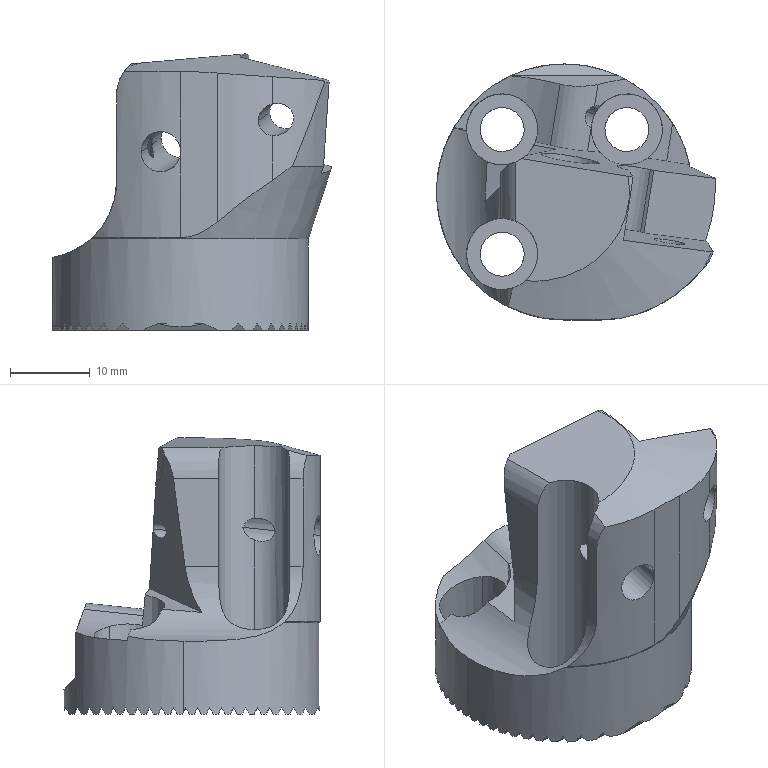NC program | Mastercam | posted with a generic post
Lines 5249 to 6702 of 7888:
(4 FEMR |TOOL - 6|DIA. OFF. - 6|LEN. - 6|TOOL DIA. - 4.)
N652 T6 M6
N654 G0 G54 G90 X24.079 Y12.972 C9. B-84. S3500 M3
N656 G43 H6 Z56.807
N658 Z7.807
N660 G1 Z6.607 F2000.
N662 G41 D6 X23.527 Y12.824 F400.
N664 G3 X23.484 Y12.769 I.014 J-.055
N666 X23.486 Y12.754 I.057
N668 G1 X23.917 Y11.146
N670 G2 X23.987 Y10.616 I-1.98 J-.53
N672 X23.616 Y9.44 I-2.05
N674 G1 X23.314 Y9.009
N676 G3 X23.196 Y8.636 I.533 J-.373
N678 X23.847 Y7.985 I.651
N680 X24.379 Y8.263 J.651
N682 G1 X24.681 Y8.694
N684 G2 X26.182 Y9.56 I1.679 J-1.176
N686 G1 X27.875 Y9.709
N688 G3 X27.926 Y9.765 I-.005 J.056
N690 G1 Y9.77
N692 G40 X27.877 Y10.34
N694 X24.079 Y12.972
N696 Z6.407 F2000.
N698 G41 D6 X23.527 Y12.824 F400.
N700 G3 X23.484 Y12.769 I.014 J-.055
N702 X23.486 Y12.754 I.057
N704 G1 X23.917 Y11.146
N706 G2 X23.987 Y10.616 I-1.98 J-.53
N708 X23.616 Y9.44 I-2.05
N710 G1 X23.314 Y9.009
N712 G3 X23.196 Y8.636 I.533 J-.373
N714 X23.847 Y7.985 I.651
N716 X24.379 Y8.263 J.651
N718 G1 X24.681 Y8.694
N720 G2 X26.182 Y9.56 I1.679 J-1.176
N722 G1 X27.875 Y9.709
N724 G3 X27.926 Y9.765 I-.005 J.056
N726 G1 Y9.77
N728 G40 X27.877 Y10.34
N730 X24.079 Y12.972
N732 Z6.207 F2000.
N734 G41 D6 X23.527 Y12.824 F400.
N736 G3 X23.484 Y12.769 I.014 J-.055
N738 X23.486 Y12.754 I.057
N740 G1 X23.917 Y11.146
N742 G2 X23.987 Y10.616 I-1.98 J-.53
N744 X23.616 Y9.44 I-2.05
N746 G1 X23.314 Y9.009
N748 G3 X23.196 Y8.636 I.533 J-.373
N750 X23.847 Y7.985 I.651
N752 X24.379 Y8.263 J.651
N754 G1 X24.681 Y8.694
N756 G2 X26.182 Y9.56 I1.679 J-1.176
N758 G1 X27.875 Y9.709
N760 G3 X27.926 Y9.765 I-.005 J.056
N762 G1 Y9.77
N764 G40 X27.877 Y10.34
N766 X24.079 Y12.972
N768 Z6.007 F2000.
N770 G41 D6 X23.527 Y12.824 F400.
N772 G3 X23.484 Y12.769 I.014 J-.055
N774 X23.486 Y12.754 I.057
N776 G1 X23.917 Y11.146
N778 G2 X23.987 Y10.616 I-1.98 J-.53
N780 X23.616 Y9.44 I-2.05
N782 G1 X23.314 Y9.009
N784 G3 X23.196 Y8.636 I.533 J-.373
N786 X23.847 Y7.985 I.651
N788 X24.379 Y8.263 J.651
N790 G1 X24.681 Y8.694
N792 G2 X26.182 Y9.56 I1.679 J-1.176
N794 G1 X27.875 Y9.709
N796 G3 X27.926 Y9.765 I-.005 J.056
N798 G1 Y9.77
N800 G40 X27.877 Y10.34
N802 X24.079 Y12.972
N804 Z5.807 F2000.
N806 G41 D6 X23.527 Y12.824 F400.
N808 G3 X23.484 Y12.769 I.014 J-.055
N810 X23.486 Y12.754 I.057
N812 G1 X23.917 Y11.146
N814 G2 X23.987 Y10.616 I-1.98 J-.53
N816 X23.616 Y9.44 I-2.05
N818 G1 X23.314 Y9.009
N820 G3 X23.196 Y8.636 I.533 J-.373
N822 X23.847 Y7.985 I.651
N824 X24.379 Y8.263 J.651
N826 G1 X24.681 Y8.694
N828 G2 X26.182 Y9.56 I1.679 J-1.176
N830 G1 X27.875 Y9.709
N832 G3 X27.926 Y9.765 I-.005 J.056
N834 G1 Y9.77
N836 G40 X27.877 Y10.34
N838 X24.079 Y12.972
N840 Z5.607 F2000.
N842 G41 D6 X23.527 Y12.824 F400.
N844 G3 X23.484 Y12.769 I.014 J-.055
N846 X23.486 Y12.754 I.057
N848 G1 X23.917 Y11.146
N850 G2 X23.987 Y10.616 I-1.98 J-.53
N852 X23.616 Y9.44 I-2.05
N854 G1 X23.314 Y9.009
N856 G3 X23.196 Y8.636 I.533 J-.373
N858 X23.847 Y7.985 I.651
N860 X24.379 Y8.263 J.651
N862 G1 X24.681 Y8.694
N864 G2 X26.182 Y9.56 I1.679 J-1.176
N866 G1 X27.875 Y9.709
N868 G3 X27.926 Y9.765 I-.005 J.056
N870 G1 Y9.77
N872 G40 X27.877 Y10.34
N874 X24.079 Y12.972
N876 Z5.407 F2000.
N878 G41 D6 X23.527 Y12.824 F400.
N880 G3 X23.484 Y12.769 I.014 J-.055
N882 X23.486 Y12.754 I.057
N884 G1 X23.917 Y11.146
N886 G2 X23.987 Y10.616 I-1.98 J-.53
N888 X23.616 Y9.44 I-2.05
N890 G1 X23.314 Y9.009
N892 G3 X23.196 Y8.636 I.533 J-.373
N894 X23.847 Y7.985 I.651
N896 X24.379 Y8.263 J.651
N898 G1 X24.681 Y8.694
N900 G2 X26.182 Y9.56 I1.679 J-1.176
N902 G1 X27.875 Y9.709
N904 G3 X27.926 Y9.765 I-.005 J.056
N906 G1 Y9.77
N908 G40 X27.877 Y10.34
N910 X24.079 Y12.972
N912 Z5.207 F2000.
N914 G41 D6 X23.527 Y12.824 F400.
N916 G3 X23.484 Y12.769 I.014 J-.055
N918 X23.486 Y12.754 I.057
N920 G1 X23.917 Y11.146
N922 G2 X23.987 Y10.616 I-1.98 J-.53
N924 X23.616 Y9.44 I-2.05
N926 G1 X23.314 Y9.009
N928 G3 X23.196 Y8.636 I.533 J-.373
N930 X23.847 Y7.985 I.651
N932 X24.379 Y8.263 J.651
N934 G1 X24.681 Y8.694
N936 G2 X26.182 Y9.56 I1.679 J-1.176
N938 G1 X27.875 Y9.709
N940 G3 X27.926 Y9.765 I-.005 J.056
N942 G1 Y9.77
N944 G40 X27.877 Y10.34
N946 X24.079 Y12.972
N948 Z5.007 F2000.
N950 G41 D6 X23.527 Y12.824 F400.
N952 G3 X23.484 Y12.769 I.014 J-.055
N954 X23.486 Y12.754 I.057
N956 G1 X23.917 Y11.146
N958 G2 X23.987 Y10.616 I-1.98 J-.53
N960 X23.616 Y9.44 I-2.05
N962 G1 X23.314 Y9.009
N964 G3 X23.196 Y8.636 I.533 J-.373
N966 X23.847 Y7.985 I.651
N968 X24.379 Y8.263 J.651
N970 G1 X24.681 Y8.694
N972 G2 X26.182 Y9.56 I1.679 J-1.176
N974 G1 X27.875 Y9.709
N976 G3 X27.926 Y9.765 I-.005 J.056
N978 G1 Y9.77
N980 G40 X27.877 Y10.34
N982 X24.079 Y12.972
N984 Z4.807 F2000.
N986 G41 D6 X23.527 Y12.824 F400.
N988 G3 X23.484 Y12.769 I.014 J-.055
N990 X23.486 Y12.754 I.057
N992 G1 X23.917 Y11.146
N994 G2 X23.987 Y10.616 I-1.98 J-.53
N996 X23.616 Y9.44 I-2.05
N998 G1 X23.314 Y9.009
N1000 G3 X23.196 Y8.636 I.533 J-.373
N1002 X23.847 Y7.985 I.651
N1004 X24.379 Y8.263 J.651
N1006 G1 X24.681 Y8.694
N1008 G2 X26.182 Y9.56 I1.679 J-1.176
N1010 G1 X27.875 Y9.709
N1012 G3 X27.926 Y9.765 I-.005 J.056
N1014 G1 Y9.77
N1016 G40 X27.877 Y10.34
N1018 X24.079 Y12.972
N1020 Z4.607 F2000.
N1022 G41 D6 X23.527 Y12.824 F400.
N1024 G3 X23.484 Y12.769 I.014 J-.055
N1026 X23.486 Y12.754 I.057
N1028 G1 X23.917 Y11.146
N1030 G2 X23.987 Y10.616 I-1.98 J-.53
N1032 X23.616 Y9.44 I-2.05
N1034 G1 X23.314 Y9.009
N1036 G3 X23.196 Y8.636 I.533 J-.373
N1038 X23.847 Y7.985 I.651
N1040 X24.379 Y8.263 J.651
N1042 G1 X24.681 Y8.694
N1044 G2 X26.182 Y9.56 I1.679 J-1.176
N1046 G1 X27.875 Y9.709
N1048 G3 X27.926 Y9.765 I-.005 J.056
N1050 G1 Y9.77
N1052 G40 X27.877 Y10.34
N1054 X24.079 Y12.972
N1056 Z4.407 F2000.
N1058 G41 D6 X23.527 Y12.824 F400.
N1060 G3 X23.484 Y12.769 I.014 J-.055
N1062 X23.486 Y12.754 I.057
N1064 G1 X23.917 Y11.146
N1066 G2 X23.987 Y10.616 I-1.98 J-.53
N1068 X23.616 Y9.44 I-2.05
N1070 G1 X23.314 Y9.009
N1072 G3 X23.196 Y8.636 I.533 J-.373
N1074 X23.847 Y7.985 I.651
N1076 X24.379 Y8.263 J.651
N1078 G1 X24.681 Y8.694
N1080 G2 X26.182 Y9.56 I1.679 J-1.176
N1082 G1 X27.875 Y9.709
N1084 G3 X27.926 Y9.765 I-.005 J.056
N1086 G1 Y9.77
N1088 G40 X27.877 Y10.34
N1090 X24.079 Y12.972
N1092 Z4.207 F2000.
N1094 G41 D6 X23.527 Y12.824 F400.
N1096 G3 X23.484 Y12.769 I.014 J-.055
N1098 X23.486 Y12.754 I.057
N1100 G1 X23.917 Y11.146
N1102 G2 X23.987 Y10.616 I-1.98 J-.53
N1104 X23.616 Y9.44 I-2.05
N1106 G1 X23.314 Y9.009
N1108 G3 X23.196 Y8.636 I.533 J-.373
N1110 X23.847 Y7.985 I.651
N1112 X24.379 Y8.263 J.651
N1114 G1 X24.681 Y8.694
N1116 G2 X26.182 Y9.56 I1.679 J-1.176
N1118 G1 X27.875 Y9.709
N1120 G3 X27.926 Y9.765 I-.005 J.056
N1122 G1 Y9.77
N1124 G40 X27.877 Y10.34
N1126 X24.079 Y12.972
N1128 Z4.007 F2000.
N1130 G41 D6 X23.527 Y12.824 F400.
N1132 G3 X23.484 Y12.769 I.014 J-.055
N1134 X23.486 Y12.754 I.057
N1136 G1 X23.917 Y11.146
N1138 G2 X23.987 Y10.616 I-1.98 J-.53
N1140 X23.616 Y9.44 I-2.05
N1142 G1 X23.314 Y9.009
N1144 G3 X23.196 Y8.636 I.533 J-.373
N1146 X23.847 Y7.985 I.651
N1148 X24.379 Y8.263 J.651
N1150 G1 X24.681 Y8.694
N1152 G2 X26.182 Y9.56 I1.679 J-1.176
N1154 G1 X27.875 Y9.709
N1156 G3 X27.926 Y9.765 I-.005 J.056
N1158 G1 Y9.77
N1160 G40 X27.877 Y10.34
N1162 X24.079 Y12.972
N1164 Z3.807 F2000.
N1166 G41 D6 X23.527 Y12.824 F400.
N1168 G3 X23.484 Y12.769 I.014 J-.055
N1170 X23.486 Y12.754 I.057
N1172 G1 X23.917 Y11.146
N1174 G2 X23.987 Y10.616 I-1.98 J-.53
N1176 X23.616 Y9.44 I-2.05
N1178 G1 X23.314 Y9.009
N1180 G3 X23.196 Y8.636 I.533 J-.373
N1182 X23.847 Y7.985 I.651
N1184 X24.379 Y8.263 J.651
N1186 G1 X24.681 Y8.694
N1188 G2 X26.182 Y9.56 I1.679 J-1.176
N1190 G1 X27.875 Y9.709
N1192 G3 X27.926 Y9.765 I-.005 J.056
N1194 G1 Y9.77
N1196 G40 X27.877 Y10.34
N1198 X24.079 Y12.972
N1200 Z3.607 F2000.
N1202 G41 D6 X23.527 Y12.824 F400.
N1204 G3 X23.484 Y12.769 I.014 J-.055
N1206 X23.486 Y12.754 I.057
N1208 G1 X23.917 Y11.146
N1210 G2 X23.987 Y10.616 I-1.98 J-.53
N1212 X23.616 Y9.44 I-2.05
N1214 G1 X23.314 Y9.009
N1216 G3 X23.196 Y8.636 I.533 J-.373
N1218 X23.847 Y7.985 I.651
N1220 X24.379 Y8.263 J.651
N1222 G1 X24.681 Y8.694
N1224 G2 X26.182 Y9.56 I1.679 J-1.176
N1226 G1 X27.875 Y9.709
N1228 G3 X27.926 Y9.765 I-.005 J.056
N1230 G1 Y9.77
N1232 G40 X27.877 Y10.34
N1234 X24.079 Y12.972
N1236 Z3.407 F2000.
N1238 G41 D6 X23.527 Y12.824 F400.
N1240 G3 X23.484 Y12.769 I.014 J-.055
N1242 X23.486 Y12.754 I.057
N1244 G1 X23.917 Y11.146
N1246 G2 X23.987 Y10.616 I-1.98 J-.53
N1248 X23.616 Y9.44 I-2.05
N1250 G1 X23.314 Y9.009
N1252 G3 X23.196 Y8.636 I.533 J-.373
N1254 X23.847 Y7.985 I.651
N1256 X24.379 Y8.263 J.651
N1258 G1 X24.681 Y8.694
N1260 G2 X26.182 Y9.56 I1.679 J-1.176
N1262 G1 X27.875 Y9.709
N1264 G3 X27.926 Y9.765 I-.005 J.056
N1266 G1 Y9.77
N1268 G40 X27.877 Y10.34
N1270 X24.079 Y12.972
N1272 Z3.207 F2000.
N1274 G41 D6 X23.527 Y12.824 F400.
N1276 G3 X23.484 Y12.769 I.014 J-.055
N1278 X23.486 Y12.754 I.057
N1280 G1 X23.917 Y11.146
N1282 G2 X23.987 Y10.616 I-1.98 J-.53
N1284 X23.616 Y9.44 I-2.05
N1286 G1 X23.314 Y9.009
N1288 G3 X23.196 Y8.636 I.533 J-.373
N1290 X23.847 Y7.985 I.651
N1292 X24.379 Y8.263 J.651
N1294 G1 X24.681 Y8.694
N1296 G2 X26.182 Y9.56 I1.679 J-1.176
N1298 G1 X27.875 Y9.709
N1300 G3 X27.926 Y9.765 I-.005 J.056
N1302 G1 Y9.77
N1304 G40 X27.877 Y10.34
N1306 X24.079 Y12.972
N1308 Z3.007 F2000.
N1310 G41 D6 X23.527 Y12.824 F400.
N1312 G3 X23.484 Y12.769 I.014 J-.055
N1314 X23.486 Y12.754 I.057
N1316 G1 X23.917 Y11.146
N1318 G2 X23.987 Y10.616 I-1.98 J-.53
N1320 X23.616 Y9.44 I-2.05
N1322 G1 X23.314 Y9.009
N1324 G3 X23.196 Y8.636 I.533 J-.373
N1326 X23.847 Y7.985 I.651
N1328 X24.379 Y8.263 J.651
N1330 G1 X24.681 Y8.694
N1332 G2 X26.182 Y9.56 I1.679 J-1.176
N1334 G1 X27.875 Y9.709
N1336 G3 X27.926 Y9.765 I-.005 J.056
N1338 G1 Y9.77
N1340 G40 X27.877 Y10.34
N1342 X24.079 Y12.972
N1344 Z2.807 F2000.
N1346 G41 D6 X23.527 Y12.824 F400.
N1348 G3 X23.484 Y12.769 I.014 J-.055
N1350 X23.486 Y12.754 I.057
N1352 G1 X23.917 Y11.146
N1354 G2 X23.987 Y10.616 I-1.98 J-.53
N1356 X23.616 Y9.44 I-2.05
N1358 G1 X23.314 Y9.009
N1360 G3 X23.196 Y8.636 I.533 J-.373
N1362 X23.847 Y7.985 I.651
N1364 X24.379 Y8.263 J.651
N1366 G1 X24.681 Y8.694
N1368 G2 X26.182 Y9.56 I1.679 J-1.176
N1370 G1 X27.875 Y9.709
N1372 G3 X27.926 Y9.765 I-.005 J.056
N1374 G1 Y9.77
N1376 G40 X27.877 Y10.34
N1378 X24.079 Y12.972
N1380 Z2.607 F2000.
N1382 G41 D6 X23.527 Y12.824 F400.
N1384 G3 X23.484 Y12.769 I.014 J-.055
N1386 X23.486 Y12.754 I.057
N1388 G1 X23.917 Y11.146
N1390 G2 X23.987 Y10.616 I-1.98 J-.53
N1392 X23.616 Y9.44 I-2.05
N1394 G1 X23.314 Y9.009
N1396 G3 X23.196 Y8.636 I.533 J-.373
N1398 X23.847 Y7.985 I.651
N1400 X24.379 Y8.263 J.651
N1402 G1 X24.681 Y8.694
N1404 G2 X26.182 Y9.56 I1.679 J-1.176
N1406 G1 X27.875 Y9.709
N1408 G3 X27.926 Y9.765 I-.005 J.056
N1410 G1 Y9.77
N1412 G40 X27.877 Y10.34
N1414 X24.079 Y12.972
N1416 Z2.407 F2000.
N1418 G41 D6 X23.527 Y12.824 F400.
N1420 G3 X23.484 Y12.769 I.014 J-.055
N1422 X23.486 Y12.754 I.057
N1424 G1 X23.917 Y11.146
N1426 G2 X23.987 Y10.616 I-1.98 J-.53
N1428 X23.616 Y9.44 I-2.05
N1430 G1 X23.314 Y9.009
N1432 G3 X23.196 Y8.636 I.533 J-.373
N1434 X23.847 Y7.985 I.651
N1436 X24.379 Y8.263 J.651
N1438 G1 X24.681 Y8.694
N1440 G2 X26.182 Y9.56 I1.679 J-1.176
N1442 G1 X27.875 Y9.709
N1444 G3 X27.926 Y9.765 I-.005 J.056
N1446 G1 Y9.77
N1448 G40 X27.877 Y10.34
N1450 X24.079 Y12.972
N1452 Z2.207 F2000.
N1454 G41 D6 X23.527 Y12.824 F400.
N1456 G3 X23.484 Y12.769 I.014 J-.055
N1458 X23.486 Y12.754 I.057
N1460 G1 X23.917 Y11.146
N1462 G2 X23.987 Y10.616 I-1.98 J-.53
N1464 X23.616 Y9.44 I-2.05
N1466 G1 X23.314 Y9.009
N1468 G3 X23.196 Y8.636 I.533 J-.373
N1470 X23.847 Y7.985 I.651
N1472 X24.379 Y8.263 J.651
N1474 G1 X24.681 Y8.694
N1476 G2 X26.182 Y9.56 I1.679 J-1.176
N1478 G1 X27.875 Y9.709
N1480 G3 X27.926 Y9.765 I-.005 J.056
N1482 G1 Y9.77
N1484 G40 X27.877 Y10.34
N1486 X24.079 Y12.972
N1488 Z2.007 F2000.
N1490 G41 D6 X23.527 Y12.824 F400.
N1492 G3 X23.484 Y12.769 I.014 J-.055
N1494 X23.486 Y12.754 I.057
N1496 G1 X23.917 Y11.146
N1498 G2 X23.987 Y10.616 I-1.98 J-.53
N1500 X23.616 Y9.44 I-2.05
N1502 G1 X23.314 Y9.009
N1504 G3 X23.196 Y8.636 I.533 J-.373
N1506 X23.847 Y7.985 I.651
N1508 X24.379 Y8.263 J.651
N1510 G1 X24.681 Y8.694
N1512 G2 X26.182 Y9.56 I1.679 J-1.176
N1514 G1 X27.875 Y9.709
N1516 G3 X27.926 Y9.765 I-.005 J.056
N1518 G1 Y9.77
N1520 G40 X27.877 Y10.34
N1522 X24.079 Y12.972
N1524 Z1.807 F2000.
N1526 G41 D6 X23.527 Y12.824 F400.
N1528 G3 X23.484 Y12.769 I.014 J-.055
N1530 X23.486 Y12.754 I.057
N1532 G1 X23.917 Y11.146
N1534 G2 X23.987 Y10.616 I-1.98 J-.53
N1536 X23.616 Y9.44 I-2.05
N1538 G1 X23.314 Y9.009
N1540 G3 X23.196 Y8.636 I.533 J-.373
N1542 X23.847 Y7.985 I.651
N1544 X24.379 Y8.263 J.651
N1546 G1 X24.681 Y8.694
N1548 G2 X26.182 Y9.56 I1.679 J-1.176
N1550 G1 X27.875 Y9.709
N1552 G3 X27.926 Y9.765 I-.005 J.056
N1554 G1 Y9.77
N1556 G40 X27.877 Y10.34
N1558 X24.079 Y12.972
N1560 Z1.607 F2000.
N1562 G41 D6 X23.527 Y12.824 F400.
N1564 G3 X23.484 Y12.769 I.014 J-.055
N1566 X23.486 Y12.754 I.057
N1568 G1 X23.917 Y11.146
N1570 G2 X23.987 Y10.616 I-1.98 J-.53
N1572 X23.616 Y9.44 I-2.05
N1574 G1 X23.314 Y9.009
N1576 G3 X23.196 Y8.636 I.533 J-.373
N1578 X23.847 Y7.985 I.651
N1580 X24.379 Y8.263 J.651
N1582 G1 X24.681 Y8.694
N1584 G2 X26.182 Y9.56 I1.679 J-1.176
N1586 G1 X27.875 Y9.709
N1588 G3 X27.926 Y9.765 I-.005 J.056
N1590 G1 Y9.77
N1592 G40 X27.877 Y10.34
N1594 X24.079 Y12.972
N1596 Z1.407 F2000.
N1598 G41 D6 X23.527 Y12.824 F400.
N1600 G3 X23.484 Y12.769 I.014 J-.055
N1602 X23.486 Y12.754 I.057
N1604 G1 X23.917 Y11.146
N1606 G2 X23.987 Y10.616 I-1.98 J-.53
N1608 X23.616 Y9.44 I-2.05
N1610 G1 X23.314 Y9.009
N1612 G3 X23.196 Y8.636 I.533 J-.373
N1614 X23.847 Y7.985 I.651
N1616 X24.379 Y8.263 J.651
N1618 G1 X24.681 Y8.694
N1620 G2 X26.182 Y9.56 I1.679 J-1.176
N1622 G1 X27.875 Y9.709
N1624 G3 X27.926 Y9.765 I-.005 J.056
N1626 G1 Y9.77
N1628 G40 X27.877 Y10.34
N1630 X24.079 Y12.972
N1632 Z1.207 F2000.
N1634 G41 D6 X23.527 Y12.824 F400.
N1636 G3 X23.484 Y12.769 I.014 J-.055
N1638 X23.486 Y12.754 I.057
N1640 G1 X23.917 Y11.146
N1642 G2 X23.987 Y10.616 I-1.98 J-.53
N1644 X23.616 Y9.44 I-2.05
N1646 G1 X23.314 Y9.009
N1648 G3 X23.196 Y8.636 I.533 J-.373
N1650 X23.847 Y7.985 I.651
N1652 X24.379 Y8.263 J.651
N1654 G1 X24.681 Y8.694
N1656 G2 X26.182 Y9.56 I1.679 J-1.176
N1658 G1 X27.875 Y9.709
N1660 G3 X27.926 Y9.765 I-.005 J.056
N1662 G1 Y9.77
N1664 G40 X27.877 Y10.34
N1666 X24.079 Y12.972
N1668 Z1.007 F2000.
N1670 G41 D6 X23.527 Y12.824 F400.
N1672 G3 X23.484 Y12.769 I.014 J-.055
N1674 X23.486 Y12.754 I.057
N1676 G1 X23.917 Y11.146
N1678 G2 X23.987 Y10.616 I-1.98 J-.53
N1680 X23.616 Y9.44 I-2.05
N1682 G1 X23.314 Y9.009
N1684 G3 X23.196 Y8.636 I.533 J-.373
N1686 X23.847 Y7.985 I.651
N1688 X24.379 Y8.263 J.651
N1690 G1 X24.681 Y8.694
N1692 G2 X26.182 Y9.56 I1.679 J-1.176
N1694 G1 X27.875 Y9.709
N1696 G3 X27.926 Y9.765 I-.005 J.056
N1698 G1 Y9.77
N1700 G40 X27.877 Y10.34
N1702 X24.079 Y12.972
N1704 Z.807 F2000.
N1706 G41 D6 X23.527 Y12.824 F400.
N1708 G3 X23.484 Y12.769 I.014 J-.055
N1710 X23.486 Y12.754 I.057
N1712 G1 X23.917 Y11.146
N1714 G2 X23.987 Y10.616 I-1.98 J-.53
N1716 X23.616 Y9.44 I-2.05
N1718 G1 X23.314 Y9.009
N1720 G3 X23.196 Y8.636 I.533 J-.373
N1722 X23.847 Y7.985 I.651
N1724 X24.379 Y8.263 J.651
N1726 G1 X24.681 Y8.694
N1728 G2 X26.182 Y9.56 I1.679 J-1.176
N1730 G1 X27.875 Y9.709
N1732 G3 X27.926 Y9.765 I-.005 J.056
N1734 G1 Y9.77
N1736 G40 X27.877 Y10.34
N1738 X24.079 Y12.972
N1740 Z.607 F2000.
N1742 G41 D6 X23.527 Y12.824 F400.
N1744 G3 X23.484 Y12.769 I.014 J-.055
N1746 X23.486 Y12.754 I.057
N1748 G1 X23.917 Y11.146
N1750 G2 X23.987 Y10.616 I-1.98 J-.53
N1752 X23.616 Y9.44 I-2.05
N1754 G1 X23.314 Y9.009
N1756 G3 X23.196 Y8.636 I.533 J-.373
N1758 X23.847 Y7.985 I.651
N1760 X24.379 Y8.263 J.651
N1762 G1 X24.681 Y8.694
N1764 G2 X26.182 Y9.56 I1.679 J-1.176
N1766 G1 X27.875 Y9.709
N1768 G3 X27.926 Y9.765 I-.005 J.056
N1770 G1 Y9.77
N1772 G40 X27.877 Y10.34
N1774 X24.079 Y12.972
N1776 Z.407 F2000.
N1778 G41 D6 X23.527 Y12.824 F400.
N1780 G3 X23.484 Y12.769 I.014 J-.055
N1782 X23.486 Y12.754 I.057
N1784 G1 X23.917 Y11.146
N1786 G2 X23.987 Y10.616 I-1.98 J-.53
N1788 X23.616 Y9.44 I-2.05
N1790 G1 X23.314 Y9.009
N1792 G3 X23.196 Y8.636 I.533 J-.373
N1794 X23.847 Y7.985 I.651
N1796 X24.379 Y8.263 J.651
N1798 G1 X24.681 Y8.694
N1800 G2 X26.182 Y9.56 I1.679 J-1.176
N1802 G1 X27.875 Y9.709
N1804 G3 X27.926 Y9.765 I-.005 J.056
N1806 G1 Y9.77
N1808 G40 X27.877 Y10.34
N1810 X24.079 Y12.972
N1812 Z.207 F2000.
N1814 G41 D6 X23.527 Y12.824 F400.
N1816 G3 X23.484 Y12.769 I.014 J-.055
N1818 X23.486 Y12.754 I.057
N1820 G1 X23.917 Y11.146
N1822 G2 X23.987 Y10.616 I-1.98 J-.53
N1824 X23.616 Y9.44 I-2.05
N1826 G1 X23.314 Y9.009
N1828 G3 X23.196 Y8.636 I.533 J-.373
N1830 X23.847 Y7.985 I.651
N1832 X24.379 Y8.263 J.651
N1834 G1 X24.681 Y8.694
N1836 G2 X26.182 Y9.56 I1.679 J-1.176
N1838 G1 X27.875 Y9.709
N1840 G3 X27.926 Y9.765 I-.005 J.056
N1842 G1 Y9.77
N1844 G40 X27.877 Y10.34
N1846 X24.079 Y12.972
N1848 Z.007 F2000.
N1850 G41 D6 X23.527 Y12.824 F400.
N1852 G3 X23.484 Y12.769 I.014 J-.055
N1854 X23.486 Y12.754 I.057
N1856 G1 X23.917 Y11.146
N1858 G2 X23.987 Y10.616 I-1.98 J-.53
N1860 X23.616 Y9.44 I-2.05
N1862 G1 X23.314 Y9.009
N1864 G3 X23.196 Y8.636 I.533 J-.373
N1866 X23.847 Y7.985 I.651
N1868 X24.379 Y8.263 J.651
N1870 G1 X24.681 Y8.694
N1872 G2 X26.182 Y9.56 I1.679 J-1.176
N1874 G1 X27.875 Y9.709
N1876 G3 X27.926 Y9.765 I-.005 J.056
N1878 G1 Y9.77
N1880 G40 X27.877 Y10.34
N1882 X24.079 Y12.972
N1884 Z-.193 F2000.
N1886 G41 D6 X23.527 Y12.824 F400.
N1888 G3 X23.484 Y12.769 I.014 J-.055
N1890 X23.486 Y12.754 I.057
N1892 G1 X23.917 Y11.146
N1894 G2 X23.987 Y10.616 I-1.98 J-.53
N1896 X23.616 Y9.44 I-2.05
N1898 G1 X23.314 Y9.009
N1900 G3 X23.196 Y8.636 I.533 J-.373
N1902 X23.847 Y7.985 I.651
N1904 X24.379 Y8.263 J.651
N1906 G1 X24.681 Y8.694
N1908 G2 X26.182 Y9.56 I1.679 J-1.176
N1910 G1 X27.875 Y9.709
N1912 G3 X27.926 Y9.765 I-.005 J.056
N1914 G1 Y9.77
N1916 G40 X27.877 Y10.34
N1918 X24.079 Y12.972
N1920 Z-.393 F2000.
N1922 G41 D6 X23.527 Y12.824 F400.
N1924 G3 X23.484 Y12.769 I.014 J-.055
N1926 X23.486 Y12.754 I.057
N1928 G1 X23.917 Y11.146
N1930 G2 X23.987 Y10.616 I-1.98 J-.53
N1932 X23.616 Y9.44 I-2.05
N1934 G1 X23.314 Y9.009
N1936 G3 X23.196 Y8.636 I.533 J-.373
N1938 X23.847 Y7.985 I.651
N1940 X24.379 Y8.263 J.651
N1942 G1 X24.681 Y8.694
N1944 G2 X26.182 Y9.56 I1.679 J-1.176
N1946 G1 X27.875 Y9.709
N1948 G3 X27.926 Y9.765 I-.005 J.056
N1950 G1 Y9.77
N1952 G40 X27.877 Y10.34
N1954 X24.079 Y12.972
N1956 Z-.593 F2000.
N1958 G41 D6 X23.527 Y12.824 F400.
N1960 G3 X23.484 Y12.769 I.014 J-.055
N1962 X23.486 Y12.754 I.057
N1964 G1 X23.917 Y11.146
N1966 G2 X23.987 Y10.616 I-1.98 J-.53
N1968 X23.616 Y9.44 I-2.05
N1970 G1 X23.314 Y9.009
N1972 G3 X23.196 Y8.636 I.533 J-.373
N1974 X23.847 Y7.985 I.651
N1976 X24.379 Y8.263 J.651
N1978 G1 X24.681 Y8.694
N1980 G2 X26.182 Y9.56 I1.679 J-1.176
N1982 G1 X27.875 Y9.709
N1984 G3 X27.926 Y9.765 I-.005 J.056
N1986 G1 Y9.77
N1988 G40 X27.877 Y10.34
N1990 X24.079 Y12.972
N1992 Z-.793 F2000.
N1994 G41 D6 X23.527 Y12.824 F400.
N1996 G3 X23.484 Y12.769 I.014 J-.055
N1998 X23.486 Y12.754 I.057
N2000 G1 X23.917 Y11.146
N2002 G2 X23.987 Y10.616 I-1.98 J-.53
N2004 X23.616 Y9.44 I-2.05
N2006 G1 X23.314 Y9.009
N2008 G3 X23.196 Y8.636 I.533 J-.373
N2010 X23.847 Y7.985 I.651
N2012 X24.379 Y8.263 J.651
N2014 G1 X24.681 Y8.694
N2016 G2 X26.182 Y9.56 I1.679 J-1.176
N2018 G1 X27.875 Y9.709
N2020 G3 X27.926 Y9.765 I-.005 J.056
N2022 G1 Y9.77
N2024 G40 X27.877 Y10.34
N2026 X24.079 Y12.972
N2028 Z-.993 F2000.
N2030 G41 D6 X23.527 Y12.824 F400.
N2032 G3 X23.484 Y12.769 I.014 J-.055
N2034 X23.486 Y12.754 I.057
N2036 G1 X23.917 Y11.146
N2038 G2 X23.987 Y10.616 I-1.98 J-.53
N2040 X23.616 Y9.44 I-2.05
N2042 G1 X23.314 Y9.009
N2044 G3 X23.196 Y8.636 I.533 J-.373
N2046 X23.847 Y7.985 I.651
N2048 X24.379 Y8.263 J.651
N2050 G1 X24.681 Y8.694
N2052 G2 X26.182 Y9.56 I1.679 J-1.176
N2054 G1 X27.875 Y9.709
N2056 G3 X27.926 Y9.765 I-.005 J.056
N2058 G1 Y9.77
N2060 G40 X27.877 Y10.34
N2062 X24.079 Y12.972
N2064 Z-1.193 F2000.
N2066 G41 D6 X23.527 Y12.824 F400.
N2068 G3 X23.484 Y12.769 I.014 J-.055
N2070 X23.486 Y12.754 I.057
N2072 G1 X23.917 Y11.146
N2074 G2 X23.987 Y10.616 I-1.98 J-.53
N2076 X23.616 Y9.44 I-2.05
N2078 G1 X23.314 Y9.009
N2080 G3 X23.196 Y8.636 I.533 J-.373
N2082 X23.847 Y7.985 I.651
N2084 X24.379 Y8.263 J.651
N2086 G1 X24.681 Y8.694
N2088 G2 X26.182 Y9.56 I1.679 J-1.176
N2090 G1 X27.875 Y9.709
N2092 G3 X27.926 Y9.765 I-.005 J.056
N2094 G1 Y9.77
N2096 G40 X27.877 Y10.34
N2098 G0 Z56.807
N2100 Z56.889
N2102 X23.57 Y-.384
N2104 Z7.889
N2106 G1 Z6.889 F2000.
N2108 G41 D6 Y-1.384 F400.
N2110 G3 X23.87 Y-1.684 I.3
N2112 X25.57 Y.016 Z6.814 J1.7
N2114 X23.87 Y1.716 Z6.739 I-1.7
N2116 X22.17 Y.016 Z6.664 J-1.7
N2118 X23.87 Y-1.684 Z6.589 I1.7
N2120 X25.57 Y.016 Z6.514 J1.7
N2122 X23.87 Y1.716 Z6.439 I-1.7
N2124 X22.17 Y.016 Z6.364 J-1.7
N2126 X23.87 Y-1.684 Z6.289 I1.7
N2128 X25.57 Y.016 Z6.214 J1.7
N2130 X23.87 Y1.716 Z6.139 I-1.7
N2132 X22.17 Y.016 Z6.064 J-1.7
N2134 X23.87 Y-1.684 Z5.989 I1.7
N2136 X25.57 Y.016 Z5.914 J1.7
N2138 X23.87 Y1.716 Z5.839 I-1.7
N2140 X22.17 Y.016 Z5.764 J-1.7
N2142 X23.87 Y-1.684 Z5.689 I1.7
N2144 X25.57 Y.016 Z5.614 J1.7
N2146 X23.87 Y1.716 Z5.539 I-1.7
N2148 X22.17 Y.016 Z5.464 J-1.7
N2150 X23.87 Y-1.684 Z5.389 I1.7
N2152 X25.57 Y.016 Z5.314 J1.7
N2154 X23.87 Y1.716 Z5.239 I-1.7
N2156 X22.17 Y.016 Z5.164 J-1.7
N2158 X23.87 Y-1.684 Z5.089 I1.7
N2160 X25.57 Y.016 Z5.014 J1.7
N2162 X23.87 Y1.716 Z4.939 I-1.7
N2164 X22.17 Y.016 Z4.864 J-1.7
N2166 X23.87 Y-1.684 Z4.789 I1.7
N2168 X25.57 Y.016 Z4.714 J1.7
N2170 X23.87 Y1.716 Z4.639 I-1.7
N2172 X22.17 Y.016 Z4.564 J-1.7
N2174 X23.87 Y-1.684 Z4.489 I1.7
N2176 X25.57 Y.016 Z4.414 J1.7
N2178 X23.87 Y1.716 Z4.339 I-1.7
N2180 X22.17 Y.016 Z4.264 J-1.7
N2182 X23.87 Y-1.684 Z4.189 I1.7
N2184 X25.57 Y.016 Z4.114 J1.7
N2186 X23.87 Y1.716 Z4.039 I-1.7
N2188 X22.17 Y.016 Z3.964 J-1.7
N2190 X23.87 Y-1.684 Z3.889 I1.7
N2192 X25.57 Y.016 Z3.814 J1.7
N2194 X23.87 Y1.716 Z3.739 I-1.7
N2196 X22.17 Y.016 Z3.664 J-1.7
N2198 X23.87 Y-1.684 Z3.589 I1.7
N2200 X25.57 Y.016 Z3.514 J1.7
N2202 X23.87 Y1.716 Z3.439 I-1.7
N2204 X22.17 Y.016 Z3.364 J-1.7
N2206 X23.87 Y-1.684 Z3.289 I1.7
N2208 X25.57 Y.016 Z3.214 J1.7
N2210 X23.87 Y1.716 Z3.139 I-1.7
N2212 X22.17 Y.016 Z3.064 J-1.7
N2214 X23.87 Y-1.684 Z2.989 I1.7
N2216 X25.57 Y.016 Z2.914 J1.7
N2218 X23.87 Y1.716 Z2.839 I-1.7
N2220 X22.17 Y.016 Z2.764 J-1.7
N2222 X23.87 Y-1.684 Z2.689 I1.7
N2224 X25.57 Y.016 J1.7
N2226 X23.87 Y1.716 I-1.7
N2228 X22.17 Y.016 J-1.7
N2230 X23.87 Y-1.684 I1.7
N2232 X24.362 Y-1.611 J1.7
N2234 X24.575 Y-1.324 I-.087 J.287
N2236 X24.563 Y-1.237 I-.3
N2238 G1 G40 X24.273 Y-.28
N2240 G0 Z56.889
N2242 M5
N2244 G0 G28 G91 Z0.
N2246 G28 C0. B0.
N2248 M01
N2250 G0 G17 G40 G80 G90 G94 G98
N2252 G0 G28 G91 Z0.
(4 FEMF |TOOL - 7|DIA. OFF. - 7|LEN. - 7|TOOL DIA. - 4.)
N2254 T7 M6
N2256 G0 G54 G90 X28.968 Y24.169 C9. B-84. S3500 M3
N2258 G43 H7 Z56.807
N2260 Z7.807
N2262 G1 Z-1.273 F2000.
N2264 G41 D7 X27.037 Y23.652 F400.
N2266 G3 X26.814 Y23.362 I.077 J-.29
N2268 X26.824 Y23.284 I.3
N2270 G1 X27.083 Y22.318
N2272 X28.839 Y15.766
N2274 X35.518 Y16.35
N2276 X36.514 Y16.437
N2278 G3 X36.788 Y16.736 I-.026 J.299
N2280 X36.787 Y16.762 I-.3
N2282 G1 G40 X36.612 Y18.754
N2284 X27.037 Y23.652
N2286 G41 D7 X25.105 Y23.134
N2288 G3 X24.882 Y22.844 I.077 J-.29
N2290 X24.893 Y22.767 I.3
N2292 G1 X25.151 Y21.801
N2294 X27.342 Y13.627
N2296 X35.692 Y14.358
N2298 X36.688 Y14.445
N2300 G3 X36.962 Y14.744 I-.026 J.299
N2302 X36.961 Y14.77 I-.3
N2304 G1 G40 X36.787 Y16.762
N2306 X25.105 Y23.134
N2308 G41 D7 X23.173 Y22.617
N2310 G3 X22.951 Y22.327 I.078 J-.29
N2312 X22.961 Y22.249 I.3
N2314 G1 X23.22 Y21.283
N2316 X25.801 Y11.651
N2318 G2 X25.841 Y11.484 I-3.864 J-1.035
N2320 X26.012 Y11.503 I.519 J-3.966
N2322 G1 X35.866 Y12.365
N2324 X36.862 Y12.452
N2326 G3 X37.136 Y12.751 I-.026 J.299
N2328 X37.135 Y12.777 I-.3
N2330 G1 G40 X36.961 Y14.77
N2332 X23.173 Y22.617
N2334 G41 D7 X21.241 Y22.099
N2336 G3 X21.019 Y21.809 I.078 J-.29
N2338 X21.029 Y21.731 I.3
N2340 G1 X21.288 Y20.766
N2342 X23.869 Y11.133
N2344 G2 X23.937 Y10.616 I-1.932 J-.517
N2346 X23.575 Y9.468 I-2.
N2348 G1 X23.273 Y9.037
N2350 G3 X23.147 Y8.636 I.574 J-.401
N2352 X23.847 Y7.936 I.7
N2354 X24.42 Y8.234 J.7
N2356 G1 X24.722 Y8.665
N2358 G2 X26.186 Y9.511 I1.638 J-1.147
N2360 G1 X36.041 Y10.373
N2362 X37.037 Y10.46
N2364 G3 X37.311 Y10.759 I-.026 J.299
N2366 X37.309 Y10.785 I-.3
N2368 G1 G40 X37.135 Y12.777
N2370 G0 Z56.807
N2372 C9.182 B-83.33
N2374 X21.183 Y20.806
N2376 Z49.997
N2378 Z.997
N2380 G1 Z-.003 F2000.
N2382 G41 D7 X21.701 Y18.874 F400.
N2384 X23.782 Y11.119
N2386 G40 X24.3 Y9.188
N2388 G0 Z49.997
N2390 C9.697 B-84.06
N2392 X24.189 Y9.283
N2394 Z49.77
N2396 Z.77
N2398 G1 Z-.23 F2000.
N2400 G41 D7 X26.181 Y9.459 F400.
N2402 X34.284 Y10.179
N2404 G40 X36.276 Y10.355
N2406 G0 Z49.77
N2408 M5
N2410 G0 G28 G91 Z0.
N2412 G28 C0. B0.
N2414 M01
N2416 G0 G17 G40 G80 G90 G94 G98
N2418 G0 G28 G91 Z0.
(12 FEMF |TOOL - 9|DIA. OFF. - 9|LEN. - 9|TOOL DIA. - 12.)
N2420 T9 M6
N2422 G0 G54 G90 X28.587 Y-10.574 C0. B0. S3500 M3
N2424 G43 H9 Z84.732
N2426 Z35.732
N2428 G1 Z9.532 F2000.
N2430 G41 D9 X25.961 Y-9.123 F600.
N2432 G3 X25.526 Y-9.011 I-.435 J-.788
N2434 X24.738 Y-9.476 J-.9
N2436 G2 X14.23 Y-19.701 I-22.123 J12.223
N2438 X4.58 Y-22.05 I-9.65 J18.651
N2440 G1 X0.
N2442 G2 X-21.717 Y-3.816 J22.05
N2444 G3 X-22.604 Y-3.071 I-.887 J-.156
N2446 X-22.759 Y-3.085 J-.901
N2448 G1 G40 X-25.714 Y-3.605
N2450 G0 Z59.532
N2452 X28.587 Y-10.574
N2454 Z35.732
N2456 G1 Z9.532 F2000.
N2458 G41 D9 X25.961 Y-9.123 F600.
N2460 G3 X25.526 Y-9.011 I-.435 J-.788
N2462 X24.738 Y-9.476 J-.9
N2464 G2 X14.23 Y-19.701 I-22.123 J12.223
N2466 X4.58 Y-22.05 I-9.65 J18.651
N2468 G1 X0.
N2470 G2 X-21.717 Y-3.816 J22.05
N2472 G3 X-22.604 Y-3.071 I-.887 J-.156
N2474 X-22.759 Y-3.085 J-.901
N2476 G1 G40 X-25.714 Y-3.605
N2478 G0 Z84.732
N2480 C9. B-84.
N2482 X14.411 Y26.729
N2484 Z57.439
N2486 Z8.439
N2488 G1 Z7.439 F2000.
N2490 G41 D9 Y16.729 F600.
N2492 Y12.021
N2494 G3 X16.506 Y5.563 I11.
N2496 G2 X18.411 Y-.308 I-8.095 J-5.871
N2498 X16.506 Y-6.179 I-10.
N2500 G3 X14.437 Y-11.887 I8.903 J-6.457
N2502 G1 Y-13.455
N2504 G40 Y-23.455
N2506 G0 Z57.439
N2508 Z66.
N2510 X10.536 Y15.764
N2512 C0. B-90.
N2514 Z17.
N2516 G1 Z14.5 F2000.
N2518 G41 D9 Y6.764 F600.
N2520 Y-6.764
N2522 G40 Y-15.764
N2524 G0 Z66.
N2526 B-45.
N2528 X-12.96
N2530 Z64.496
N2532 Z15.496
N2534 G1 Z13.496 F2000.
N2536 G41 D9 Y-6.764 F600.
N2538 Y6.764
N2540 G40 Y15.764
N2542 G0 Z64.496
N2544 Z68.131
N2546 X9.673
N2548 B-70.
N2550 Z19.131
N2552 G1 Z17.131 F2000.
N2554 G41 D9 Y6.764 F600.
N2556 Y-6.764
N2558 G40 Y-15.764
N2560 G0 Z68.131
N2562 Z70.698
N2564 X-14.847 Y-20.312
N2566 B-270.
N2568 Z21.698
N2570 G1 Z-9.302 F2000.
N2572 G41 D9 X-15.005 Y-17.316 F600.
N2574 G3 X-18.5 Y-14. I-3.495 J-.184
N2576 G1 X-29.407
N2578 G2 X-37.971 Y-9.904 J11.
N2580 G1 X-39.117 Y-8.481
N2582 X-40.873 Y11.591
N2584 G40 X-40.96 Y12.587
N2586 G0 Z70.698
N2588 M5
N2590 G0 G28 G91 Z0.
N2592 G28 B0.
N2594 M01
N2596 G0 G17 G40 G80 G90 G94 G98
N2598 G0 G28 G91 Z0.
(30 BNOS |TOOL - 10|DIA. OFF. - 10|LEN. - 10|TOOL DIA. - 30.)
N2600 T10 M6
N2602 G0 G54 G90 X23.411 Y36.729 C9. B-84. S3500 M3
N2604 G43 H10 Z57.689
N2606 Z8.689
N2608 G1 Z6.689 F2000.
N2610 G41 D10 Y16.729 F400.
N2612 Y12.021
N2614 G3 X23.792 Y10.847 I2.
N2616 G2 X27.411 Y-.308 I-15.381 J-11.155
N2618 X23.792 Y-11.462 I-19.
N2620 G3 X23.437 Y-12.318 I1.616 J-1.173
N2622 G1 Y-12.798
N2624 X23.579 Y-14.41
N2626 X23.509 Y-18.171
N2628 G40 X23.23 Y-33.168
N2630 G0 Z57.689
N2632 M5
N2634 G0 G28 G91 Z0.
N2636 G28 C0. B0.
N2638 M01
N2640 G0 G17 G40 G80 G90 G94 G98
N2642 G0 G28 G91 Z0.
(6 SPD |TOOL - 12|DIA. OFF. - 12|LEN. - 12|TOOL DIA. - 6.)
N2644 T12 M6
N2646 G0 G54 G90 X7.75 Y0. C0. B-90. S2000 M3
N2648 G43 H12 Z64.5
N2650 G81 G98 Z13.5 R15.5 F100.
N2652 G80
N2654 C9. B-84.
N2656 X22.578 Y-4.815
N2658 Z56.689
N2660 G81 G98 Z5.689 R7.689 F100.
N2662 G80
N2664 X23.87 Y.016
N2666 Z52.704
N2668 G81 G98 Z1.704 R3.704 F100.
N2670 G80
N2672 X27.461 Y13.957
N2674 Z48.707
N2676 G81 G98 Z-2.293 R-.293 F100.
N2678 G80
N2680 M5
N2682 G0 G28 G91 Z0.
N2684 G28 C0. B0.
N2686 M01
N2688 G0 G17 G40 G80 G90 G94 G98
N2690 G0 G28 G91 Z0.
(4.3 DR |TOOL - 3|DIA. OFF. - 3|LEN. - 3|TOOL DIA. - 4.3)
N2692 T3 M6
N2694 G0 G54 G90 X23.87 Y.016 C9. B-84. S2500 M3
N2696 G43 H3 Z52.704
N2698 G83 G98 Z-15.796 R3.704 Q4. F100.
N2700 G80
N2702 M5
N2704 G0 G28 G91 Z0.
N2706 G28 C0. B0.
N2708 M01
N2710 G0 G17 G40 G80 G90 G94 G98
N2712 G0 G28 G91 Z0.
(3.3 DR |TOOL - 13|DIA. OFF. - 13|LEN. - 13|TOOL DIA. - 3.3)
N2714 T13 M6
N2716 G0 G54 G90 X27.461 Y13.957 C9. B-84. S3000 M3
N2718 G43 H13 Z48.707
N2720 G83 G98 Z-12.293 R-.293 Q4. F60.
N2722 G80
N2724 Z64.5
N2726 X7.75 Y0.
N2728 C0. B-90.
N2730 G83 G98 Z2.5 R15.5 Q4. F60.
N2732 G80
N2734 M5
N2736 G0 G28 G91 Z0.
N2738 G28 B0.
N2740 M01
N2742 G0 G17 G40 G80 G90 G94 G98
N2744 G0 G28 G91 Z0.
(2 DR |TOOL - 1|DIA. OFF. - 1|LEN. - 1|TOOL DIA. - 2.)
N2746 T1 M6
N2748 G0 G54 G90 X22.578 Y-4.815 C9. B-84. S3000 M3
N2750 G43 H1 Z56.689
N2752 G81 G98 Z1.089 R7.689 F60.
N2754 G80
N2756 M5
N2758 G0 G28 G91 Z0.
N2760 G28 C0. B0.
N2762 M01
N2764 G0 G17 G40 G80 G90 G94 G98
N2766 G0 G28 G91 Z0.
(4 FEM |TOOL - 11|DIA. OFF. - 11|LEN. - 11|TOOL DIA. - 4.)
N2768 T11 M6
N2770 G0 G54 G90 X27.461 Y-13.957 C189. B-96. S2000 M3
N2772 G43 H11 Z60.649
N2774 G81 G98 Z6.649 R11.649 F100.
N2776 G80
N2778 M5
N2780 G0 G28 G91 Z0.
N2782 G28 C0. B0.
N2784 M01
N2786 G0 G17 G40 G80 G90 G94 G98
N2788 G0 G28 G91 Z0.
(5.5 FL |TOOL - 18|DIA. OFF. - 18|LEN. - 18|TOOL DIA. - 5.5)
N2790 T18 M6
N2792 G0 G54 G90 X23.87 Y-.016 C189. B-96. S1000 M3
N2794 G43 H18 Z63.92
N2796 G81 G98 Z8.92 R14.92 F100.
N2798 G80
N2800 M5
N2802 G0 G28 G91 Z0.
N2804 G28 C0. B0.
N2806 M01
N2808 G0 G17 G40 G80 G90 G94 G98
N2810 G0 G28 G91 Z0.
(6 SPD |TOOL - 12|DIA. OFF. - 12|LEN. - 12|TOOL DIA. - 6.)
N2812 T12 M6
N2814 G0 G54 G90 X23.87 Y.016 C9. B-84. S2000 M3
N2816 G43 H12 Z52.704
N2818 G81 G98 Z.104 R3.704 F200.
N2820 G80
N2822 X27.461 Y13.957
N2824 Z48.707
N2826 G81 G98 Z-3.393 R-.293 F200.
N2828 G80
N2830 Z64.5
N2832 X7.75 Y0.
N2834 C0. B-90.
N2836 G81 G98 Z12.4 R15.5 F200.
N2838 G80
N2840 M5
N2842 G0 G28 G91 Z0.
N2844 G28 B0.
N2846 M01
N2848 G0 G17 G40 G80 G90 G94 G98
N2850 G0 G28 G91 Z0.
(3.15 THML |TOOL - 14|DIA. OFF. - 14|LEN. - 14|TOOL DIA. - 3.15)
N2852 T14 M6
N2854 G0 G54 G90 X7.75 Y0. C0. B-90. S3000 M3
N2856 G43 H14 Z64.5
N2858 Z16.5
N2860 G1 Z10.8 F2000.
N2862 G41 D14 X7.98 F300.
N2864 G3 X7.75 Y.23 Z10.975 I-.23
N2866 X7.52 Y0. Z11.15 J-.23
N2868 X7.75 Y-.23 Z11.325 I.23
N2870 X7.98 Y0. Z11.5 J.23
N2872 X7.75 Y.23 Z11.675 I-.23
N2874 X7.52 Y0. Z11.85 J-.23
N2876 G1 G40 X7.75
N2878 Z12.9 F2000.
N2880 G41 D14 X7.98 F300.
N2882 G3 X7.75 Y.23 Z13.075 I-.23
N2884 X7.52 Y0. Z13.25 J-.23
N2886 X7.75 Y-.23 Z13.425 I.23
N2888 X7.98 Y0. Z13.6 J.23
N2890 X7.75 Y.23 Z13.775 I-.23
N2892 X7.52 Y0. Z13.95 J-.23
N2894 G1 G40 X7.75
N2896 Z10.8 F2000.
N2898 G41 D14 X8.045 F300.
N2900 G3 X7.75 Y.295 Z10.975 I-.295
N2902 X7.455 Y0. Z11.15 J-.295
N2904 X7.75 Y-.295 Z11.325 I.295
N2906 X8.045 Y0. Z11.5 J.295
N2908 X7.75 Y.295 Z11.675 I-.295
N2910 X7.455 Y0. Z11.85 J-.295
N2912 G1 G40 X7.75
N2914 Z12.9 F2000.
N2916 G41 D14 X8.045 F300.
N2918 G3 X7.75 Y.295 Z13.075 I-.295
N2920 X7.455 Y0. Z13.25 J-.295
N2922 X7.75 Y-.295 Z13.425 I.295
N2924 X8.045 Y0. Z13.6 J.295
N2926 X7.75 Y.295 Z13.775 I-.295
N2928 X7.455 Y0. Z13.95 J-.295
N2930 G1 G40 X7.75
N2932 Z10.8 F2000.
N2934 G41 D14 X8.11 F300.
N2936 G3 X7.75 Y.36 Z10.975 I-.36
N2938 X7.39 Y0. Z11.15 J-.36
N2940 X7.75 Y-.36 Z11.325 I.36
N2942 X8.11 Y0. Z11.5 J.36
N2944 X7.75 Y.36 Z11.675 I-.36
N2946 X7.39 Y0. Z11.85 J-.36
N2948 G1 G40 X7.75
N2950 Z12.9 F2000.
N2952 G41 D14 X8.11 F300.
N2954 G3 X7.75 Y.36 Z13.075 I-.36
N2956 X7.39 Y0. Z13.25 J-.36
N2958 X7.75 Y-.36 Z13.425 I.36
N2960 X8.11 Y0. Z13.6 J.36
N2962 X7.75 Y.36 Z13.775 I-.36
N2964 X7.39 Y0. Z13.95 J-.36
N2966 G1 G40 X7.75
N2968 Z10.8 F2000.
N2970 G41 D14 X8.175 F300.
N2972 G3 X7.75 Y.425 Z10.975 I-.425
N2974 X7.325 Y0. Z11.15 J-.425
N2976 X7.75 Y-.425 Z11.325 I.425
N2978 X8.175 Y0. Z11.5 J.425
N2980 X7.75 Y.425 Z11.675 I-.425
N2982 X7.325 Y0. Z11.85 J-.425
N2984 G1 G40 X7.75
N2986 Z12.9 F2000.
N2988 G41 D14 X8.175 F300.
N2990 G3 X7.75 Y.425 Z13.075 I-.425
N2992 X7.325 Y0. Z13.25 J-.425
N2994 X7.75 Y-.425 Z13.425 I.425
N2996 X8.175 Y0. Z13.6 J.425
N2998 X7.75 Y.425 Z13.775 I-.425
N3000 X7.325 Y0. Z13.95 J-.425
N3002 G1 G40 X7.75
N3004 G0 Z16.5
N3006 Z64.5
N3008 C9. B-84.
N3010 X27.461 Y13.957
N3012 Z48.707
N3014 Z.707
N3016 G1 Z-10.293 F2000.
N3018 G41 D14 X27.626 F300.
N3020 G3 X27.461 Y14.122 Z-10.118 I-.165
N3022 X27.296 Y13.957 Z-9.943 J-.165
N3024 X27.461 Y13.792 Z-9.768 I.165
N3026 X27.626 Y13.957 Z-9.593 J.165
N3028 X27.461 Y14.122 Z-9.418 I-.165
N3030 X27.296 Y13.957 Z-9.243 J-.165
N3032 G1 G40 X27.461
N3034 Z-8.193 F2000.
N3036 G41 D14 X27.626 F300.
N3038 G3 X27.461 Y14.122 Z-8.018 I-.165
N3040 X27.296 Y13.957 Z-7.843 J-.165
N3042 X27.461 Y13.792 Z-7.668 I.165
N3044 X27.626 Y13.957 Z-7.493 J.165
N3046 X27.461 Y14.122 Z-7.318 I-.165
N3048 X27.296 Y13.957 Z-7.143 J-.165
N3050 G1 G40 X27.461
N3052 Z-6.093 F2000.
N3054 G41 D14 X27.626 F300.
N3056 G3 X27.461 Y14.122 Z-5.918 I-.165
N3058 X27.296 Y13.957 Z-5.743 J-.165
N3060 X27.461 Y13.792 Z-5.568 I.165
N3062 X27.626 Y13.957 Z-5.393 J.165
N3064 X27.461 Y14.122 Z-5.218 I-.165
N3066 X27.296 Y13.957 Z-5.043 J-.165
N3068 G1 G40 X27.461
N3070 Z-3.993 F2000.
N3072 G41 D14 X27.626 F300.
N3074 G3 X27.461 Y14.122 Z-3.818 I-.165
N3076 X27.296 Y13.957 Z-3.643 J-.165
N3078 X27.461 Y13.792 Z-3.468 I.165
N3080 X27.626 Y13.957 Z-3.293 J.165
N3082 X27.461 Y14.122 Z-3.118 I-.165
N3084 X27.296 Y13.957 Z-2.943 J-.165
N3086 X27.461 Y13.792 Z-2.768 I.165
N3088 X27.626 Y13.957 Z-2.593 J.165
N3090 X27.461 Y14.122 Z-2.418 I-.165
N3092 X27.296 Y13.957 Z-2.243 J-.165
N3094 G1 G40 X27.461
N3096 Z-10.293 F2000.
N3098 G41 D14 X27.691 F300.
N3100 G3 X27.461 Y14.187 Z-10.118 I-.23
N3102 X27.231 Y13.957 Z-9.943 J-.23
N3104 X27.461 Y13.727 Z-9.768 I.23
N3106 X27.691 Y13.957 Z-9.593 J.23
N3108 X27.461 Y14.187 Z-9.418 I-.23
N3110 X27.231 Y13.957 Z-9.243 J-.23
N3112 G1 G40 X27.461
N3114 Z-8.193 F2000.
N3116 G41 D14 X27.691 F300.
N3118 G3 X27.461 Y14.187 Z-8.018 I-.23
N3120 X27.231 Y13.957 Z-7.843 J-.23
N3122 X27.461 Y13.727 Z-7.668 I.23
N3124 X27.691 Y13.957 Z-7.493 J.23
N3126 X27.461 Y14.187 Z-7.318 I-.23
N3128 X27.231 Y13.957 Z-7.143 J-.23
N3130 G1 G40 X27.461
N3132 Z-6.093 F2000.
N3134 G41 D14 X27.691 F300.
N3136 G3 X27.461 Y14.187 Z-5.918 I-.23
N3138 X27.231 Y13.957 Z-5.743 J-.23
N3140 X27.461 Y13.727 Z-5.568 I.23
N3142 X27.691 Y13.957 Z-5.393 J.23
N3144 X27.461 Y14.187 Z-5.218 I-.23
N3146 X27.231 Y13.957 Z-5.043 J-.23
N3148 G1 G40 X27.461
N3150 Z-3.993 F2000.
N3152 G41 D14 X27.691 F300.
N3154 G3 X27.461 Y14.187 Z-3.818 I-.23
N3156 X27.231 Y13.957 Z-3.643 J-.23
N3158 X27.461 Y13.727 Z-3.468 I.23
N3160 X27.691 Y13.957 Z-3.293 J.23
N3162 X27.461 Y14.187 Z-3.118 I-.23
N3164 X27.231 Y13.957 Z-2.943 J-.23
N3166 X27.461 Y13.727 Z-2.768 I.23
N3168 X27.691 Y13.957 Z-2.593 J.23
N3170 X27.461 Y14.187 Z-2.418 I-.23
N3172 X27.231 Y13.957 Z-2.243 J-.23
N3174 G1 G40 X27.461
N3176 Z-10.293 F2000.
N3178 G41 D14 X27.756 F300.
N3180 G3 X27.461 Y14.252 Z-10.118 I-.295
N3182 X27.166 Y13.957 Z-9.943 J-.295
N3184 X27.461 Y13.662 Z-9.768 I.295
N3186 X27.756 Y13.957 Z-9.593 J.295
N3188 X27.461 Y14.252 Z-9.418 I-.295
N3190 X27.166 Y13.957 Z-9.243 J-.295
N3192 G1 G40 X27.461
N3194 Z-8.193 F2000.
N3196 G41 D14 X27.756 F300.
N3198 G3 X27.461 Y14.252 Z-8.018 I-.295
N3200 X27.166 Y13.957 Z-7.843 J-.295
N3202 X27.461 Y13.662 Z-7.668 I.295
N3204 X27.756 Y13.957 Z-7.493 J.295
N3206 X27.461 Y14.252 Z-7.318 I-.295
N3208 X27.166 Y13.957 Z-7.143 J-.295
N3210 G1 G40 X27.461
N3212 Z-6.093 F2000.
N3214 G41 D14 X27.756 F300.
N3216 G3 X27.461 Y14.252 Z-5.918 I-.295
N3218 X27.166 Y13.957 Z-5.743 J-.295
N3220 X27.461 Y13.662 Z-5.568 I.295
N3222 X27.756 Y13.957 Z-5.393 J.295
N3224 X27.461 Y14.252 Z-5.218 I-.295
N3226 X27.166 Y13.957 Z-5.043 J-.295
N3228 G1 G40 X27.461
N3230 Z-3.993 F2000.
N3232 G41 D14 X27.756 F300.
N3234 G3 X27.461 Y14.252 Z-3.818 I-.295
N3236 X27.166 Y13.957 Z-3.643 J-.295
N3238 X27.461 Y13.662 Z-3.468 I.295
N3240 X27.756 Y13.957 Z-3.293 J.295
N3242 X27.461 Y14.252 Z-3.118 I-.295
N3244 X27.166 Y13.957 Z-2.943 J-.295
N3246 X27.461 Y13.662 Z-2.768 I.295
N3248 X27.756 Y13.957 Z-2.593 J.295
N3250 X27.461 Y14.252 Z-2.418 I-.295
N3252 X27.166 Y13.957 Z-2.243 J-.295
N3254 G1 G40 X27.461
N3256 Z-10.293 F2000.
N3258 G41 D14 X27.821 F300.
N3260 G3 X27.461 Y14.317 Z-10.118 I-.36
N3262 X27.101 Y13.957 Z-9.943 J-.36
N3264 X27.461 Y13.597 Z-9.768 I.36
N3266 X27.821 Y13.957 Z-9.593 J.36
N3268 X27.461 Y14.317 Z-9.418 I-.36
N3270 X27.101 Y13.957 Z-9.243 J-.36
N3272 G1 G40 X27.461
N3274 Z-8.193 F2000.
N3276 G41 D14 X27.821 F300.
N3278 G3 X27.461 Y14.317 Z-8.018 I-.36
N3280 X27.101 Y13.957 Z-7.843 J-.36
N3282 X27.461 Y13.597 Z-7.668 I.36
N3284 X27.821 Y13.957 Z-7.493 J.36
N3286 X27.461 Y14.317 Z-7.318 I-.36
N3288 X27.101 Y13.957 Z-7.143 J-.36
N3290 G1 G40 X27.461
N3292 Z-6.093 F2000.
N3294 G41 D14 X27.821 F300.
N3296 G3 X27.461 Y14.317 Z-5.918 I-.36
N3298 X27.101 Y13.957 Z-5.743 J-.36
N3300 X27.461 Y13.597 Z-5.568 I.36
N3302 X27.821 Y13.957 Z-5.393 J.36
N3304 X27.461 Y14.317 Z-5.218 I-.36
N3306 X27.101 Y13.957 Z-5.043 J-.36
N3308 G1 G40 X27.461
N3310 Z-3.993 F2000.
N3312 G41 D14 X27.821 F300.
N3314 G3 X27.461 Y14.317 Z-3.818 I-.36
N3316 X27.101 Y13.957 Z-3.643 J-.36
N3318 X27.461 Y13.597 Z-3.468 I.36
N3320 X27.821 Y13.957 Z-3.293 J.36
N3322 X27.461 Y14.317 Z-3.118 I-.36
N3324 X27.101 Y13.957 Z-2.943 J-.36
N3326 X27.461 Y13.597 Z-2.768 I.36
N3328 X27.821 Y13.957 Z-2.593 J.36
N3330 X27.461 Y14.317 Z-2.418 I-.36
N3332 X27.101 Y13.957 Z-2.243 J-.36
N3334 G1 G40 X27.461
N3336 Z-10.293 F2000.
N3338 G41 D14 X27.886 F300.
N3340 G3 X27.461 Y14.382 Z-10.118 I-.425
N3342 X27.036 Y13.957 Z-9.943 J-.425
N3344 X27.461 Y13.532 Z-9.768 I.425
N3346 X27.886 Y13.957 Z-9.593 J.425
N3348 X27.461 Y14.382 Z-9.418 I-.425
N3350 X27.036 Y13.957 Z-9.243 J-.425
N3352 G1 G40 X27.461
N3354 Z-8.193 F2000.
N3356 G41 D14 X27.886 F300.
N3358 G3 X27.461 Y14.382 Z-8.018 I-.425
N3360 X27.036 Y13.957 Z-7.843 J-.425
N3362 X27.461 Y13.532 Z-7.668 I.425
N3364 X27.886 Y13.957 Z-7.493 J.425
N3366 X27.461 Y14.382 Z-7.318 I-.425
N3368 X27.036 Y13.957 Z-7.143 J-.425
N3370 G1 G40 X27.461
N3372 Z-6.093 F2000.
N3374 G41 D14 X27.886 F300.
N3376 G3 X27.461 Y14.382 Z-5.918 I-.425
N3378 X27.036 Y13.957 Z-5.743 J-.425
N3380 X27.461 Y13.532 Z-5.568 I.425
N3382 X27.886 Y13.957 Z-5.393 J.425
N3384 X27.461 Y14.382 Z-5.218 I-.425
N3386 X27.036 Y13.957 Z-5.043 J-.425
N3388 G1 G40 X27.461
N3390 Z-3.993 F2000.
N3392 G41 D14 X27.886 F300.
N3394 G3 X27.461 Y14.382 Z-3.818 I-.425
N3396 X27.036 Y13.957 Z-3.643 J-.425
N3398 X27.461 Y13.532 Z-3.468 I.425
N3400 X27.886 Y13.957 Z-3.293 J.425
N3402 X27.461 Y14.382 Z-3.118 I-.425
N3404 X27.036 Y13.957 Z-2.943 J-.425
N3406 X27.461 Y13.532 Z-2.768 I.425
N3408 X27.886 Y13.957 Z-2.593 J.425
N3410 X27.461 Y14.382 Z-2.418 I-.425
N3412 X27.036 Y13.957 Z-2.243 J-.425
N3414 G1 G40 X27.461
N3416 Z-10.293 F2000.
N3418 G41 D14 X27.886 F300.
N3420 G3 X27.461 Y14.382 Z-10.118 I-.425
N3422 X27.036 Y13.957 Z-9.943 J-.425
N3424 X27.461 Y13.532 Z-9.768 I.425
N3426 X27.886 Y13.957 Z-9.593 J.425
N3428 X27.461 Y14.382 Z-9.418 I-.425
N3430 X27.036 Y13.957 Z-9.243 J-.425
N3432 G1 G40 X27.461
N3434 Z-8.193 F2000.
N3436 G41 D14 X27.886 F300.
N3438 G3 X27.461 Y14.382 Z-8.018 I-.425
N3440 X27.036 Y13.957 Z-7.843 J-.425
N3442 X27.461 Y13.532 Z-7.668 I.425
N3444 X27.886 Y13.957 Z-7.493 J.425
N3446 X27.461 Y14.382 Z-7.318 I-.425
N3448 X27.036 Y13.957 Z-7.143 J-.425
N3450 G1 G40 X27.461
N3452 Z-6.093 F2000.
N3454 G41 D14 X27.886 F300.
N3456 G3 X27.461 Y14.382 Z-5.918 I-.425
N3458 X27.036 Y13.957 Z-5.743 J-.425
N3460 X27.461 Y13.532 Z-5.568 I.425
N3462 X27.886 Y13.957 Z-5.393 J.425
N3464 X27.461 Y14.382 Z-5.218 I-.425
N3466 X27.036 Y13.957 Z-5.043 J-.425
N3468 G1 G40 X27.461
N3470 Z-3.993 F2000.
N3472 G41 D14 X27.886 F300.
N3474 G3 X27.461 Y14.382 Z-3.818 I-.425
N3476 X27.036 Y13.957 Z-3.643 J-.425
N3478 X27.461 Y13.532 Z-3.468 I.425
N3480 X27.886 Y13.957 Z-3.293 J.425
N3482 X27.461 Y14.382 Z-3.118 I-.425
N3484 X27.036 Y13.957 Z-2.943 J-.425
N3486 X27.461 Y13.532 Z-2.768 I.425
N3488 X27.886 Y13.957 Z-2.593 J.425
N3490 X27.461 Y14.382 Z-2.418 I-.425
N3492 X27.036 Y13.957 Z-2.243 J-.425
N3494 G1 G40 X27.461
N3496 G0 Z.707
N3498 Z48.707
N3500 M5
N3502 G0 G28 G91 Z0.
N3504 G28 C0. B0.
N3506 M01
N3508 G0 G17 G40 G80 G90 G94 G98
N3510 G0 G28 G91 Z0.
(M5 X 0.8 RH |TOOL - 16|DIA. OFF. - 16|LEN. - 16|TOOL DIA. - 5.)
N3512 T16 M6
N3514 G0 G54 G90 X23.87 Y.016 C9. B-84. S200 M3
N3516 G43 H16 Z52.704
N3518 G84 G98 Z-5.296 R3.704 F160.
N3520 G80
N3522 M5
N3524 G0 G28 G91 Z0.
N3526 G28 C0. B0.
N3528 M01
N3530 G0 G17 G40 G80 G90 G94 G98
N3532 G0 G28 G91 Z0.